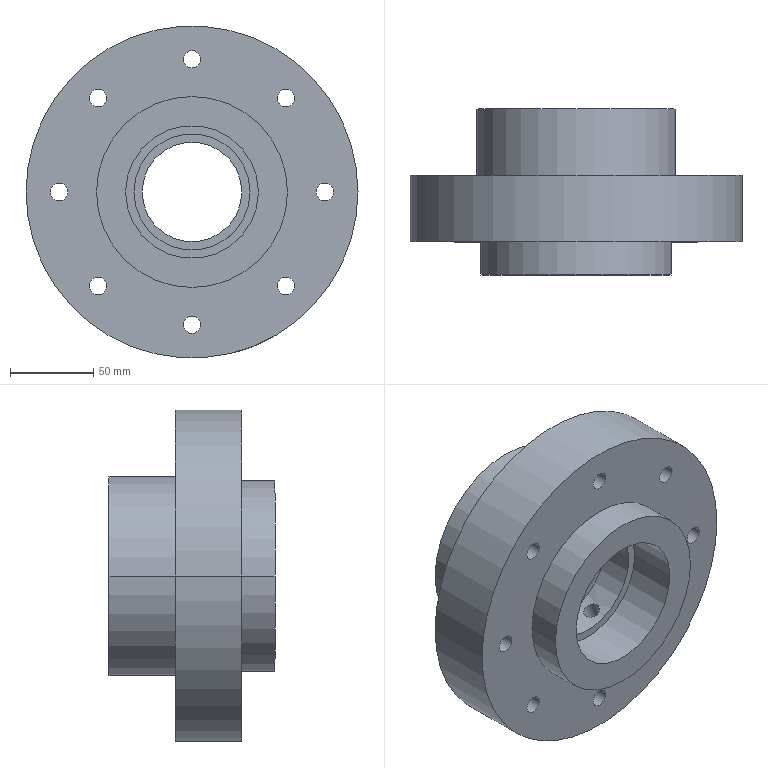Part | SolidWorks | features ICE 4, RevCut 1, Revolution 1 | 1 solid | 79 faces | box 200 x 100 x 200 mm | volume 1489766 mm3 | cylinder 56 | plane 21 | cone 2 | commonest cylinder face diameters 10.5 x16 18 x16 60 x6 70 x6 8 x2 9.882 x2